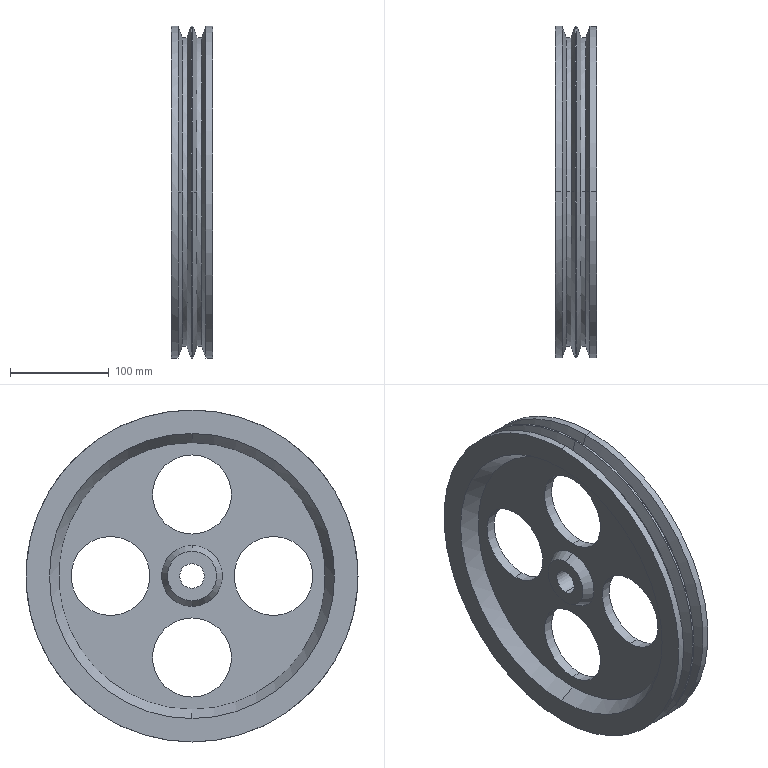Part | SolidWorks | features BaseBody 1 | 1 solid | 42 faces | box 42 x 336 x 336 mm | volume 1380304 mm3 | cylinder 20 | cone 16 | plane 6 | commonest cylinder face diameters 80 x8 336 x6 312.6 x4 25 x2
STEP:
#1=CARTESIAN_POINT('',(-5.,0.,-135.));
#2=VERTEX_POINT('',#1);
#3=CARTESIAN_POINT('',(-5.,0.,135.));
#4=VERTEX_POINT('',#3);
#5=CARTESIAN_POINT('',(-5.,0.,0.));
#6=DIRECTION('',(-1.,0.,0.));
#7=DIRECTION('',(0.,0.,1.));
#8=AXIS2_PLACEMENT_3D('',#5,#6,#7);
#9=CIRCLE('',#8,135.);
#10=EDGE_CURVE('',#2,#4,#9,.T.);
#11=ORIENTED_EDGE('',*,*,#10,.F.);
#12=CARTESIAN_POINT('',(-21.,0.,-144.238));
#13=VERTEX_POINT('',#12);
#14=CARTESIAN_POINT('',(-21.,0.,-144.238));
#15=DIRECTION('',(-0.866,0.,-0.5));
#16=VECTOR('',#15,1000.);
#17=LINE('',#14,#16);
#18=EDGE_CURVE('',#2,#13,#17,.T.);
#19=ORIENTED_EDGE('',*,*,#18,.T.);
#20=CARTESIAN_POINT('',(-21.,0.,144.238));
#21=VERTEX_POINT('',#20);
#22=CARTESIAN_POINT('',(-21.,0.,0.));
#23=DIRECTION('',(1.,0.,0.));
#24=DIRECTION('',(0.,0.,1.));
#25=AXIS2_PLACEMENT_3D('',#22,#23,#24);
#26=CIRCLE('',#25,144.238);
#27=EDGE_CURVE('',#21,#13,#26,.T.);
#28=ORIENTED_EDGE('',*,*,#27,.F.);
#29=CARTESIAN_POINT('',(-21.,0.,144.238));
#30=DIRECTION('',(-0.866,0.,0.5));
#31=VECTOR('',#30,1000.);
#32=LINE('',#29,#31);
#33=EDGE_CURVE('',#4,#21,#32,.T.);
#34=ORIENTED_EDGE('',*,*,#33,.F.);
#35=EDGE_LOOP('',(#11,#19,#28,#34));
#36=FACE_OUTER_BOUND('',#35,.T.);
#37=CARTESIAN_POINT('',(-21.,0.,0.));
#38=DIRECTION('',(-1.,0.,0.));
#39=DIRECTION('',(0.,0.,1.));
#40=AXIS2_PLACEMENT_3D('',#37,#38,#39);
#41=CONICAL_SURFACE('',#40,144.238,0.5236);
#42=ADVANCED_FACE('',(#36),#41,.F.);
#43=CARTESIAN_POINT('',(-15.,0.,-25.));
#44=VERTEX_POINT('',#43);
#45=CARTESIAN_POINT('',(-15.,0.,25.));
#46=VERTEX_POINT('',#45);
#47=CARTESIAN_POINT('',(-15.,0.,0.));
#48=DIRECTION('',(1.,0.,0.));
#49=DIRECTION('',(0.,0.,-1.));
#50=AXIS2_PLACEMENT_3D('',#47,#48,#49);
#51=CIRCLE('',#50,25.);
#52=EDGE_CURVE('',#44,#46,#51,.T.);
#53=ORIENTED_EDGE('',*,*,#52,.T.);
#54=CARTESIAN_POINT('',(-5.,0.,30.774));
#55=VERTEX_POINT('',#54);
#56=CARTESIAN_POINT('',(-5.,0.,30.774));
#57=DIRECTION('',(0.866,0.,0.5));
#58=VECTOR('',#57,1000.);
#59=LINE('',#56,#58);
#60=EDGE_CURVE('',#46,#55,#59,.T.);
#61=ORIENTED_EDGE('',*,*,#60,.T.);
#62=CARTESIAN_POINT('',(-5.,0.,-30.774));
#63=VERTEX_POINT('',#62);
#64=CARTESIAN_POINT('',(-5.,0.,0.));
#65=DIRECTION('',(1.,0.,0.));
#66=DIRECTION('',(0.,0.,-1.));
#67=AXIS2_PLACEMENT_3D('',#64,#65,#66);
#68=CIRCLE('',#67,30.774);
#69=EDGE_CURVE('',#63,#55,#68,.T.);
#70=ORIENTED_EDGE('',*,*,#69,.F.);
#71=CARTESIAN_POINT('',(-5.,0.,-30.774));
#72=DIRECTION('',(0.866,0.,-0.5));
#73=VECTOR('',#72,1000.);
#74=LINE('',#71,#73);
#75=EDGE_CURVE('',#44,#63,#74,.T.);
#76=ORIENTED_EDGE('',*,*,#75,.F.);
#77=EDGE_LOOP('',(#53,#61,#70,#76));
#78=FACE_OUTER_BOUND('',#77,.T.);
#79=CARTESIAN_POINT('',(-5.,0.,0.));
#80=DIRECTION('',(1.,0.,0.));
#81=DIRECTION('',(0.,0.,-1.));
#82=AXIS2_PLACEMENT_3D('',#79,#80,#81);
#83=CONICAL_SURFACE('',#82,30.774,0.5236);
#84=ADVANCED_FACE('',(#78),#83,.T.);
#85=CARTESIAN_POINT('',(5.,82.5,-40.));
#86=VERTEX_POINT('',#85);
#87=CARTESIAN_POINT('',(5.,82.5,40.));
#88=VERTEX_POINT('',#87);
#89=CARTESIAN_POINT('',(5.,82.5,0.));
#90=DIRECTION('',(-1.,0.,0.));
#91=DIRECTION('',(0.,0.,1.));
#92=AXIS2_PLACEMENT_3D('',#89,#90,#91);
#93=CIRCLE('',#92,40.);
#94=EDGE_CURVE('',#86,#88,#93,.T.);
#95=ORIENTED_EDGE('',*,*,#94,.F.);
#96=CARTESIAN_POINT('',(-5.,82.5,-40.));
#97=VERTEX_POINT('',#96);
#98=CARTESIAN_POINT('',(5.,82.5,-40.));
#99=DIRECTION('',(-1.,0.,0.));
#100=VECTOR('',#99,1000.);
#101=LINE('',#98,#100);
#102=EDGE_CURVE('',#86,#97,#101,.T.);
#103=ORIENTED_EDGE('',*,*,#102,.T.);
#104=CARTESIAN_POINT('',(-5.,82.5,40.));
#105=VERTEX_POINT('',#104);
#106=CARTESIAN_POINT('',(-5.,82.5,0.));
#107=DIRECTION('',(1.,0.,0.));
#108=DIRECTION('',(0.,0.,1.));
#109=AXIS2_PLACEMENT_3D('',#106,#107,#108);
#110=CIRCLE('',#109,40.);
#111=EDGE_CURVE('',#105,#97,#110,.T.);
#112=ORIENTED_EDGE('',*,*,#111,.F.);
#113=CARTESIAN_POINT('',(5.,82.5,40.));
#114=DIRECTION('',(-1.,0.,0.));
#115=VECTOR('',#114,1000.);
#116=LINE('',#113,#115);
#117=EDGE_CURVE('',#88,#105,#116,.T.);
#118=ORIENTED_EDGE('',*,*,#117,.F.);
#119=EDGE_LOOP('',(#95,#103,#112,#118));
#120=FACE_OUTER_BOUND('',#119,.T.);
#121=CARTESIAN_POINT('',(5.,82.5,0.));
#122=DIRECTION('',(-1.,0.,0.));
#123=DIRECTION('',(0.,0.,1.));
#124=AXIS2_PLACEMENT_3D('',#121,#122,#123);
#125=CYLINDRICAL_SURFACE('',#124,40.);
#126=ADVANCED_FACE('',(#120),#125,.F.);
#127=CARTESIAN_POINT('',(5.,0.,42.5));
#128=VERTEX_POINT('',#127);
#129=CARTESIAN_POINT('',(5.,0.,122.5));
#130=VERTEX_POINT('',#129);
#131=CARTESIAN_POINT('',(5.,0.,82.5));
#132=DIRECTION('',(-1.,0.,0.));
#133=DIRECTION('',(0.,0.,1.));
#134=AXIS2_PLACEMENT_3D('',#131,#132,#133);
#135=CIRCLE('',#134,40.);
#136=EDGE_CURVE('',#128,#130,#135,.T.);
#137=ORIENTED_EDGE('',*,*,#136,.F.);
#138=CARTESIAN_POINT('',(-5.,0.,42.5));
#139=VERTEX_POINT('',#138);
#140=CARTESIAN_POINT('',(5.,0.,42.5));
#141=DIRECTION('',(-1.,0.,0.));
#142=VECTOR('',#141,1000.);
#143=LINE('',#140,#142);
#144=EDGE_CURVE('',#128,#139,#143,.T.);
#145=ORIENTED_EDGE('',*,*,#144,.T.);
#146=CARTESIAN_POINT('',(-5.,0.,122.5));
#147=VERTEX_POINT('',#146);
#148=CARTESIAN_POINT('',(-5.,0.,82.5));
#149=DIRECTION('',(1.,0.,0.));
#150=DIRECTION('',(0.,0.,1.));
#151=AXIS2_PLACEMENT_3D('',#148,#149,#150);
#152=CIRCLE('',#151,40.);
#153=EDGE_CURVE('',#147,#139,#152,.T.);
#154=ORIENTED_EDGE('',*,*,#153,.F.);
#155=CARTESIAN_POINT('',(5.,0.,122.5));
#156=DIRECTION('',(-1.,0.,0.));
#157=VECTOR('',#156,1000.);
#158=LINE('',#155,#157);
#159=EDGE_CURVE('',#130,#147,#158,.T.);
#160=ORIENTED_EDGE('',*,*,#159,.F.);
#161=EDGE_LOOP('',(#137,#145,#154,#160));
#162=FACE_OUTER_BOUND('',#161,.T.);
#163=CARTESIAN_POINT('',(5.,0.,82.5));
#164=DIRECTION('',(-1.,0.,0.));
#165=DIRECTION('',(0.,0.,1.));
#166=AXIS2_PLACEMENT_3D('',#163,#164,#165);
#167=CYLINDRICAL_SURFACE('',#166,40.);
#168=ADVANCED_FACE('',(#162),#167,.F.);
#169=CARTESIAN_POINT('',(5.,-82.5,-40.));
#170=VERTEX_POINT('',#169);
#171=CARTESIAN_POINT('',(5.,-82.5,40.));
#172=VERTEX_POINT('',#171);
#173=CARTESIAN_POINT('',(5.,-82.5,0.));
#174=DIRECTION('',(-1.,0.,0.));
#175=DIRECTION('',(0.,0.,1.));
#176=AXIS2_PLACEMENT_3D('',#173,#174,#175);
#177=CIRCLE('',#176,40.);
#178=EDGE_CURVE('',#170,#172,#177,.T.);
#179=ORIENTED_EDGE('',*,*,#178,.F.);
#180=CARTESIAN_POINT('',(-5.,-82.5,-40.));
#181=VERTEX_POINT('',#180);
#182=CARTESIAN_POINT('',(5.,-82.5,-40.));
#183=DIRECTION('',(-1.,0.,0.));
#184=VECTOR('',#183,1000.);
#185=LINE('',#182,#184);
#186=EDGE_CURVE('',#170,#181,#185,.T.);
#187=ORIENTED_EDGE('',*,*,#186,.T.);
#188=CARTESIAN_POINT('',(-5.,-82.5,40.));
#189=VERTEX_POINT('',#188);
#190=CARTESIAN_POINT('',(-5.,-82.5,0.));
#191=DIRECTION('',(1.,0.,0.));
#192=DIRECTION('',(0.,0.,1.));
#193=AXIS2_PLACEMENT_3D('',#190,#191,#192);
#194=CIRCLE('',#193,40.);
#195=EDGE_CURVE('',#189,#181,#194,.T.);
#196=ORIENTED_EDGE('',*,*,#195,.F.);
#197=CARTESIAN_POINT('',(5.,-82.5,40.));
#198=DIRECTION('',(-1.,0.,0.));
#199=VECTOR('',#198,1000.);
#200=LINE('',#197,#199);
#201=EDGE_CURVE('',#172,#189,#200,.T.);
#202=ORIENTED_EDGE('',*,*,#201,.F.);
#203=EDGE_LOOP('',(#179,#187,#196,#202));
#204=FACE_OUTER_BOUND('',#203,.T.);
#205=CARTESIAN_POINT('',(5.,-82.5,0.));
#206=DIRECTION('',(-1.,0.,0.));
#207=DIRECTION('',(0.,0.,1.));
#208=AXIS2_PLACEMENT_3D('',#205,#206,#207);
#209=CYLINDRICAL_SURFACE('',#208,40.);
#210=ADVANCED_FACE('',(#204),#209,.F.);
#211=CARTESIAN_POINT('',(5.,0.,-122.5));
#212=VERTEX_POINT('',#211);
#213=CARTESIAN_POINT('',(5.,0.,-42.5));
#214=VERTEX_POINT('',#213);
#215=CARTESIAN_POINT('',(5.,0.,-82.5));
#216=DIRECTION('',(-1.,0.,0.));
#217=DIRECTION('',(0.,0.,1.));
#218=AXIS2_PLACEMENT_3D('',#215,#216,#217);
#219=CIRCLE('',#218,40.);
#220=EDGE_CURVE('',#212,#214,#219,.T.);
#221=ORIENTED_EDGE('',*,*,#220,.F.);
#222=CARTESIAN_POINT('',(-5.,0.,-122.5));
#223=VERTEX_POINT('',#222);
#224=CARTESIAN_POINT('',(5.,0.,-122.5));
#225=DIRECTION('',(-1.,0.,0.));
#226=VECTOR('',#225,1000.);
#227=LINE('',#224,#226);
#228=EDGE_CURVE('',#212,#223,#227,.T.);
#229=ORIENTED_EDGE('',*,*,#228,.T.);
#230=CARTESIAN_POINT('',(-5.,0.,-42.5));
#231=VERTEX_POINT('',#230);
#232=CARTESIAN_POINT('',(-5.,0.,-82.5));
#233=DIRECTION('',(1.,0.,0.));
#234=DIRECTION('',(0.,0.,1.));
#235=AXIS2_PLACEMENT_3D('',#232,#233,#234);
#236=CIRCLE('',#235,40.);
#237=EDGE_CURVE('',#231,#223,#236,.T.);
#238=ORIENTED_EDGE('',*,*,#237,.F.);
#239=CARTESIAN_POINT('',(5.,0.,-42.5));
#240=DIRECTION('',(-1.,0.,0.));
#241=VECTOR('',#240,1000.);
#242=LINE('',#239,#241);
#243=EDGE_CURVE('',#214,#231,#242,.T.);
#244=ORIENTED_EDGE('',*,*,#243,.F.);
#245=EDGE_LOOP('',(#221,#229,#238,#244));
#246=FACE_OUTER_BOUND('',#245,.T.);
#247=CARTESIAN_POINT('',(5.,0.,-82.5));
#248=DIRECTION('',(-1.,0.,0.));
#249=DIRECTION('',(0.,0.,1.));
#250=AXIS2_PLACEMENT_3D('',#247,#248,#249);
#251=CYLINDRICAL_SURFACE('',#250,40.);
#252=ADVANCED_FACE('',(#246),#251,.F.);
#253=CARTESIAN_POINT('',(-21.,0.,168.));
#254=VERTEX_POINT('',#253);
#255=CARTESIAN_POINT('',(-21.,0.,-168.));
#256=VERTEX_POINT('',#255);
#257=CARTESIAN_POINT('',(-21.,0.,0.));
#258=DIRECTION('',(-1.,0.,0.));
#259=DIRECTION('',(0.,0.,-1.));
#260=AXIS2_PLACEMENT_3D('',#257,#258,#259);
#261=CIRCLE('',#260,168.);
#262=EDGE_CURVE('',#254,#256,#261,.T.);
#263=ORIENTED_EDGE('',*,*,#262,.F.);
#264=CARTESIAN_POINT('',(-14.033,0.,168.));
#265=VERTEX_POINT('',#264);
#266=CARTESIAN_POINT('',(0.,0.,168.));
#267=DIRECTION('',(1.,0.,0.));
#268=VECTOR('',#267,1000.);
#269=LINE('',#266,#268);
#270=EDGE_CURVE('',#254,#265,#269,.T.);
#271=ORIENTED_EDGE('',*,*,#270,.T.);
#272=CARTESIAN_POINT('',(-14.033,168.,0.));
#273=VERTEX_POINT('',#272);
#274=CARTESIAN_POINT('',(-14.033,0.,0.));
#275=DIRECTION('',(-1.,0.,0.));
#276=DIRECTION('',(0.,0.,-1.));
#277=AXIS2_PLACEMENT_3D('',#274,#275,#276);
#278=CIRCLE('',#277,168.);
#279=EDGE_CURVE('',#265,#273,#278,.T.);
#280=ORIENTED_EDGE('',*,*,#279,.T.);
#281=CARTESIAN_POINT('',(-14.033,0.,-168.));
#282=VERTEX_POINT('',#281);
#283=CARTESIAN_POINT('',(-14.033,0.,0.));
#284=DIRECTION('',(-1.,0.,0.));
#285=DIRECTION('',(0.,0.,-1.));
#286=AXIS2_PLACEMENT_3D('',#283,#284,#285);
#287=CIRCLE('',#286,168.);
#288=EDGE_CURVE('',#273,#282,#287,.T.);
#289=ORIENTED_EDGE('',*,*,#288,.T.);
#290=CARTESIAN_POINT('',(0.,0.,-168.));
#291=DIRECTION('',(1.,0.,0.));
#292=VECTOR('',#291,1000.);
#293=LINE('',#290,#292);
#294=EDGE_CURVE('',#256,#282,#293,.T.);
#295=ORIENTED_EDGE('',*,*,#294,.F.);
#296=EDGE_LOOP('',(#263,#271,#280,#289,#295));
#297=FACE_OUTER_BOUND('',#296,.T.);
#298=CARTESIAN_POINT('',(0.,0.,0.));
#299=DIRECTION('',(1.,0.,0.));
#300=DIRECTION('',(0.,0.,-1.));
#301=AXIS2_PLACEMENT_3D('',#298,#299,#300);
#302=CYLINDRICAL_SURFACE('',#301,168.);
#303=ADVANCED_FACE('',(#297),#302,.T.);
#304=CARTESIAN_POINT('',(-15.,0.,12.5));
#305=VERTEX_POINT('',#304);
#306=CARTESIAN_POINT('',(-15.,0.,-12.5));
#307=VERTEX_POINT('',#306);
#308=CARTESIAN_POINT('',(-15.,0.,0.));
#309=DIRECTION('',(1.,0.,0.));
#310=DIRECTION('',(0.,0.,-1.));
#311=AXIS2_PLACEMENT_3D('',#308,#309,#310);
#312=CIRCLE('',#311,12.5);
#313=EDGE_CURVE('',#305,#307,#312,.T.);
#314=ORIENTED_EDGE('',*,*,#313,.F.);
#315=CARTESIAN_POINT('',(15.,0.,12.5));
#316=VERTEX_POINT('',#315);
#317=CARTESIAN_POINT('',(0.,0.,12.5));
#318=DIRECTION('',(1.,0.,0.));
#319=VECTOR('',#318,1000.);
#320=LINE('',#317,#319);
#321=EDGE_CURVE('',#305,#316,#320,.T.);
#322=ORIENTED_EDGE('',*,*,#321,.T.);
#323=CARTESIAN_POINT('',(15.,0.,-12.5));
#324=VERTEX_POINT('',#323);
#325=CARTESIAN_POINT('',(15.,0.,0.));
#326=DIRECTION('',(-1.,0.,0.));
#327=DIRECTION('',(0.,0.,-1.));
#328=AXIS2_PLACEMENT_3D('',#325,#326,#327);
#329=CIRCLE('',#328,12.5);
#330=EDGE_CURVE('',#324,#316,#329,.T.);
#331=ORIENTED_EDGE('',*,*,#330,.F.);
#332=CARTESIAN_POINT('',(0.,0.,-12.5));
#333=DIRECTION('',(1.,0.,0.));
#334=VECTOR('',#333,1000.);
#335=LINE('',#332,#334);
#336=EDGE_CURVE('',#307,#324,#335,.T.);
#337=ORIENTED_EDGE('',*,*,#336,.F.);
#338=EDGE_LOOP('',(#314,#322,#331,#337));
#339=FACE_OUTER_BOUND('',#338,.T.);
#340=CARTESIAN_POINT('',(0.,0.,0.));
#341=DIRECTION('',(1.,0.,0.));
#342=DIRECTION('',(0.,0.,-1.));
#343=AXIS2_PLACEMENT_3D('',#340,#341,#342);
#344=CYLINDRICAL_SURFACE('',#343,12.5);
#345=ADVANCED_FACE('',(#339),#344,.F.);
#346=CARTESIAN_POINT('',(15.,0.,25.));
#347=VERTEX_POINT('',#346);
#348=CARTESIAN_POINT('',(15.,0.,-25.));
#349=VERTEX_POINT('',#348);
#350=CARTESIAN_POINT('',(15.,0.,0.));
#351=DIRECTION('',(-1.,0.,0.));
#352=DIRECTION('',(0.,0.,1.));
#353=AXIS2_PLACEMENT_3D('',#350,#351,#352);
#354=CIRCLE('',#353,25.);
#355=EDGE_CURVE('',#347,#349,#354,.T.);
#356=ORIENTED_EDGE('',*,*,#355,.T.);
#357=CARTESIAN_POINT('',(5.,0.,-30.774));
#358=VERTEX_POINT('',#357);
#359=CARTESIAN_POINT('',(5.,0.,-30.774));
#360=DIRECTION('',(-0.866,0.,-0.5));
#361=VECTOR('',#360,1000.);
#362=LINE('',#359,#361);
#363=EDGE_CURVE('',#349,#358,#362,.T.);
#364=ORIENTED_EDGE('',*,*,#363,.T.);
#365=CARTESIAN_POINT('',(5.,0.,30.774));
#366=VERTEX_POINT('',#365);
#367=CARTESIAN_POINT('',(5.,0.,0.));
#368=DIRECTION('',(-1.,0.,0.));
#369=DIRECTION('',(0.,0.,1.));
#370=AXIS2_PLACEMENT_3D('',#367,#368,#369);
#371=CIRCLE('',#370,30.774);
#372=EDGE_CURVE('',#366,#358,#371,.T.);
#373=ORIENTED_EDGE('',*,*,#372,.F.);
#374=CARTESIAN_POINT('',(5.,0.,30.774));
#375=DIRECTION('',(-0.866,0.,0.5));
#376=VECTOR('',#375,1000.);
#377=LINE('',#374,#376);
#378=EDGE_CURVE('',#347,#366,#377,.T.);
#379=ORIENTED_EDGE('',*,*,#378,.F.);
#380=EDGE_LOOP('',(#356,#364,#373,#379));
#381=FACE_OUTER_BOUND('',#380,.T.);
#382=CARTESIAN_POINT('',(5.,0.,0.));
#383=DIRECTION('',(-1.,0.,0.));
#384=DIRECTION('',(0.,0.,1.));
#385=AXIS2_PLACEMENT_3D('',#382,#383,#384);
#386=CONICAL_SURFACE('',#385,30.774,0.5236);
#387=ADVANCED_FACE('',(#381),#386,.T.);
#388=CARTESIAN_POINT('',(5.,0.,135.));
#389=VERTEX_POINT('',#388);
#390=CARTESIAN_POINT('',(5.,0.,-135.));
#391=VERTEX_POINT('',#390);
#392=CARTESIAN_POINT('',(5.,0.,0.));
#393=DIRECTION('',(1.,0.,0.));
#394=DIRECTION('',(0.,0.,-1.));
#395=AXIS2_PLACEMENT_3D('',#392,#393,#394);
#396=CIRCLE('',#395,135.);
#397=EDGE_CURVE('',#389,#391,#396,.T.);
#398=ORIENTED_EDGE('',*,*,#397,.F.);
#399=CARTESIAN_POINT('',(21.,0.,144.238));
#400=VERTEX_POINT('',#399);
#401=CARTESIAN_POINT('',(21.,0.,144.238));
#402=DIRECTION('',(0.866,0.,0.5));
#403=VECTOR('',#402,1000.);
#404=LINE('',#401,#403);
#405=EDGE_CURVE('',#389,#400,#404,.T.);
#406=ORIENTED_EDGE('',*,*,#405,.T.);
#407=CARTESIAN_POINT('',(21.,0.,-144.238));
#408=VERTEX_POINT('',#407);
#409=CARTESIAN_POINT('',(21.,0.,0.));
#410=DIRECTION('',(-1.,0.,0.));
#411=DIRECTION('',(0.,0.,-1.));
#412=AXIS2_PLACEMENT_3D('',#409,#410,#411);
#413=CIRCLE('',#412,144.238);
#414=EDGE_CURVE('',#408,#400,#413,.T.);
#415=ORIENTED_EDGE('',*,*,#414,.F.);
#416=CARTESIAN_POINT('',(21.,0.,-144.238));
#417=DIRECTION('',(0.866,0.,-0.5));
#418=VECTOR('',#417,1000.);
#419=LINE('',#416,#418);
#420=EDGE_CURVE('',#391,#408,#419,.T.);
#421=ORIENTED_EDGE('',*,*,#420,.F.);
#422=EDGE_LOOP('',(#398,#406,#415,#421));
#423=FACE_OUTER_BOUND('',#422,.T.);
#424=CARTESIAN_POINT('',(21.,0.,0.));
#425=DIRECTION('',(1.,0.,0.));
#426=DIRECTION('',(0.,0.,-1.));
#427=AXIS2_PLACEMENT_3D('',#424,#425,#426);
#428=CONICAL_SURFACE('',#427,144.238,0.5236);
#429=ADVANCED_FACE('',(#423),#428,.F.);
#430=CARTESIAN_POINT('',(-10.004,0.,156.3));
#431=VERTEX_POINT('',#430);
#432=CARTESIAN_POINT('',(-10.004,156.3,0.));
#433=VERTEX_POINT('',#432);
#434=CARTESIAN_POINT('',(-10.004,0.,0.));
#435=DIRECTION('',(-1.,0.,0.));
#436=DIRECTION('',(0.,0.,1.));
#437=AXIS2_PLACEMENT_3D('',#434,#435,#436);
#438=CIRCLE('',#437,156.3);
#439=EDGE_CURVE('',#431,#433,#438,.T.);
#440=ORIENTED_EDGE('',*,*,#439,.T.);
#441=CARTESIAN_POINT('',(-14.033,168.,0.));
#442=DIRECTION('',(-0.3256,0.9455,0.));
#443=VECTOR('',#442,1000.);
#444=LINE('',#441,#443);
#445=EDGE_CURVE('',#433,#273,#444,.T.);
#446=ORIENTED_EDGE('',*,*,#445,.T.);
#447=ORIENTED_EDGE('',*,*,#279,.F.);
#448=CARTESIAN_POINT('',(-14.033,-168.,0.));
#449=VERTEX_POINT('',#448);
#450=CARTESIAN_POINT('',(-14.033,0.,0.));
#451=DIRECTION('',(-1.,0.,0.));
#452=DIRECTION('',(0.,0.,-1.));
#453=AXIS2_PLACEMENT_3D('',#450,#451,#452);
#454=CIRCLE('',#453,168.);
#455=EDGE_CURVE('',#449,#265,#454,.T.);
#456=ORIENTED_EDGE('',*,*,#455,.F.);
#457=CARTESIAN_POINT('',(-10.004,-156.3,0.));
#458=VERTEX_POINT('',#457);
#459=CARTESIAN_POINT('',(-14.033,-168.,0.));
#460=DIRECTION('',(-0.3256,-0.9455,0.));
#461=VECTOR('',#460,1000.);
#462=LINE('',#459,#461);
#463=EDGE_CURVE('',#458,#449,#462,.T.);
#464=ORIENTED_EDGE('',*,*,#463,.F.);
#465=CARTESIAN_POINT('',(-10.004,0.,0.));
#466=DIRECTION('',(-1.,0.,0.));
#467=DIRECTION('',(0.,0.,1.));
#468=AXIS2_PLACEMENT_3D('',#465,#466,#467);
#469=CIRCLE('',#468,156.3);
#470=EDGE_CURVE('',#458,#431,#469,.T.);
#471=ORIENTED_EDGE('',*,*,#470,.T.);
#472=EDGE_LOOP('',(#440,#446,#447,#456,#464,#471));
#473=FACE_OUTER_BOUND('',#472,.T.);
#474=CARTESIAN_POINT('',(-14.033,0.,0.));
#475=DIRECTION('',(-1.,0.,0.));
#476=DIRECTION('',(0.,-1.,0.));
#477=AXIS2_PLACEMENT_3D('',#474,#475,#476);
#478=CONICAL_SURFACE('',#477,168.,1.239);
#479=ADVANCED_FACE('',(#473),#478,.T.);
#480=CARTESIAN_POINT('',(-4.996,0.,156.3));
#481=VERTEX_POINT('',#480);
#482=CARTESIAN_POINT('',(-4.996,0.,-156.3));
#483=VERTEX_POINT('',#482);
#484=CARTESIAN_POINT('',(-4.996,0.,0.));
#485=DIRECTION('',(-1.,0.,0.));
#486=DIRECTION('',(0.,0.,1.));
#487=AXIS2_PLACEMENT_3D('',#484,#485,#486);
#488=CIRCLE('',#487,156.3);
#489=EDGE_CURVE('',#481,#483,#488,.T.);
#490=ORIENTED_EDGE('',*,*,#489,.T.);
#491=CARTESIAN_POINT('',(-10.004,0.,-156.3));
#492=VERTEX_POINT('',#491);
#493=CARTESIAN_POINT('',(-15.,0.,-156.3));
#494=DIRECTION('',(-1.,0.,0.));
#495=VECTOR('',#494,1000.);
#496=LINE('',#493,#495);
#497=EDGE_CURVE('',#483,#492,#496,.T.);
#498=ORIENTED_EDGE('',*,*,#497,.T.);
#499=CARTESIAN_POINT('',(-10.004,0.,0.));
#500=DIRECTION('',(-1.,0.,0.));
#501=DIRECTION('',(0.,0.,1.));
#502=AXIS2_PLACEMENT_3D('',#499,#500,#501);
#503=CIRCLE('',#502,156.3);
#504=EDGE_CURVE('',#433,#492,#503,.T.);
#505=ORIENTED_EDGE('',*,*,#504,.F.);
#506=ORIENTED_EDGE('',*,*,#439,.F.);
#507=CARTESIAN_POINT('',(-15.,0.,156.3));
#508=DIRECTION('',(-1.,0.,0.));
#509=VECTOR('',#508,1000.);
#510=LINE('',#507,#509);
#511=EDGE_CURVE('',#481,#431,#510,.T.);
#512=ORIENTED_EDGE('',*,*,#511,.F.);
#513=EDGE_LOOP('',(#490,#498,#505,#506,#512));
#514=FACE_OUTER_BOUND('',#513,.T.);
#515=CARTESIAN_POINT('',(-15.,0.,0.));
#516=DIRECTION('',(-1.,0.,0.));
#517=DIRECTION('',(0.,0.,1.));
#518=AXIS2_PLACEMENT_3D('',#515,#516,#517);
#519=CYLINDRICAL_SURFACE('',#518,156.3);
#520=ADVANCED_FACE('',(#514),#519,.T.);
#521=CARTESIAN_POINT('',(14.033,0.,-168.));
#522=VERTEX_POINT('',#521);
#523=CARTESIAN_POINT('',(14.033,0.,168.));
#524=VERTEX_POINT('',#523);
#525=CARTESIAN_POINT('',(14.033,0.,0.));
#526=DIRECTION('',(1.,0.,0.));
#527=DIRECTION('',(0.,0.,-1.));
#528=AXIS2_PLACEMENT_3D('',#525,#526,#527);
#529=CIRCLE('',#528,168.);
#530=EDGE_CURVE('',#522,#524,#529,.T.);
#531=ORIENTED_EDGE('',*,*,#530,.T.);
#532=CARTESIAN_POINT('',(21.,0.,168.));
#533=VERTEX_POINT('',#532);
#534=CARTESIAN_POINT('',(0.,0.,168.));
#535=DIRECTION('',(1.,0.,0.));
#536=VECTOR('',#535,1000.);
#537=LINE('',#534,#536);
#538=EDGE_CURVE('',#524,#533,#537,.T.);
#539=ORIENTED_EDGE('',*,*,#538,.T.);
#540=CARTESIAN_POINT('',(21.,0.,-168.));
#541=VERTEX_POINT('',#540);
#542=CARTESIAN_POINT('',(21.,0.,0.));
#543=DIRECTION('',(1.,0.,0.));
#544=DIRECTION('',(0.,0.,-1.));
#545=AXIS2_PLACEMENT_3D('',#542,#543,#544);
#546=CIRCLE('',#545,168.);
#547=EDGE_CURVE('',#541,#533,#546,.T.);
#548=ORIENTED_EDGE('',*,*,#547,.F.);
#549=CARTESIAN_POINT('',(0.,0.,-168.));
#550=DIRECTION('',(1.,0.,0.));
#551=VECTOR('',#550,1000.);
#552=LINE('',#549,#551);
#553=EDGE_CURVE('',#522,#541,#552,.T.);
#554=ORIENTED_EDGE('',*,*,#553,.F.);
#555=EDGE_LOOP('',(#531,#539,#548,#554));
#556=FACE_OUTER_BOUND('',#555,.T.);
#557=CARTESIAN_POINT('',(0.,0.,0.));
#558=DIRECTION('',(1.,0.,0.));
#559=DIRECTION('',(0.,0.,-1.));
#560=AXIS2_PLACEMENT_3D('',#557,#558,#559);
#561=CYLINDRICAL_SURFACE('',#560,168.);
#562=ADVANCED_FACE('',(#556),#561,.T.);
#563=ORIENTED_EDGE('',*,*,#489,.F.);
#564=CARTESIAN_POINT('',(-0.967,0.,168.));
#565=VERTEX_POINT('',#564);
#566=CARTESIAN_POINT('',(-0.967,0.,168.));
#567=DIRECTION('',(0.3256,0.,0.9455));
#568=VECTOR('',#567,1000.);
#569=LINE('',#566,#568);
#570=EDGE_CURVE('',#481,#565,#569,.T.);
#571=ORIENTED_EDGE('',*,*,#570,.T.);
#572=CARTESIAN_POINT('',(-0.967,0.,-168.));
#573=VERTEX_POINT('',#572);
#574=CARTESIAN_POINT('',(-0.967,0.,0.));
#575=DIRECTION('',(-1.,0.,0.));
#576=DIRECTION('',(0.,0.,-1.));
#577=AXIS2_PLACEMENT_3D('',#574,#575,#576);
#578=CIRCLE('',#577,168.);
#579=EDGE_CURVE('',#565,#573,#578,.T.);
#580=ORIENTED_EDGE('',*,*,#579,.T.);
#581=CARTESIAN_POINT('',(-0.967,0.,-168.));
#582=DIRECTION('',(0.3256,0.,-0.9455));
#583=VECTOR('',#582,1000.);
#584=LINE('',#581,#583);
#585=EDGE_CURVE('',#483,#573,#584,.T.);
#586=ORIENTED_EDGE('',*,*,#585,.F.);
#587=EDGE_LOOP('',(#563,#571,#580,#586));
#588=FACE_OUTER_BOUND('',#587,.T.);
#589=CARTESIAN_POINT('',(-0.967,0.,0.));
#590=DIRECTION('',(1.,0.,0.));
#591=DIRECTION('',(0.,0.,-1.));
#592=AXIS2_PLACEMENT_3D('',#589,#590,#591);
#593=CONICAL_SURFACE('',#592,168.,1.239);
#594=ADVANCED_FACE('',(#588),#593,.T.);
#595=CARTESIAN_POINT('',(10.004,0.,-156.3));
#596=VERTEX_POINT('',#595);
#597=CARTESIAN_POINT('',(10.004,0.,156.3));
#598=VERTEX_POINT('',#597);
#599=CARTESIAN_POINT('',(10.004,0.,0.));
#600=DIRECTION('',(1.,0.,0.));
#601=DIRECTION('',(0.,0.,-1.));
#602=AXIS2_PLACEMENT_3D('',#599,#600,#601);
#603=CIRCLE('',#602,156.3);
#604=EDGE_CURVE('',#596,#598,#603,.T.);
#605=ORIENTED_EDGE('',*,*,#604,.T.);
#606=CARTESIAN_POINT('',(14.033,0.,168.));
#607=DIRECTION('',(0.3256,0.,0.9455));
#608=VECTOR('',#607,1000.);
#609=LINE('',#606,#608);
#610=EDGE_CURVE('',#598,#524,#609,.T.);
#611=ORIENTED_EDGE('',*,*,#610,.T.);
#612=ORIENTED_EDGE('',*,*,#530,.F.);
#613=CARTESIAN_POINT('',(14.033,0.,-168.));
#614=DIRECTION('',(0.3256,0.,-0.9455));
#615=VECTOR('',#614,1000.);
#616=LINE('',#613,#615);
#617=EDGE_CURVE('',#596,#522,#616,.T.);
#618=ORIENTED_EDGE('',*,*,#617,.F.);
#619=EDGE_LOOP('',(#605,#611,#612,#618));
#620=FACE_OUTER_BOUND('',#619,.T.);
#621=CARTESIAN_POINT('',(14.033,0.,0.));
#622=DIRECTION('',(1.,0.,0.));
#623=DIRECTION('',(0.,0.,-1.));
#624=AXIS2_PLACEMENT_3D('',#621,#622,#623);
#625=CONICAL_SURFACE('',#624,168.,1.239);
#626=ADVANCED_FACE('',(#620),#625,.T.);
#627=ORIENTED_EDGE('',*,*,#579,.F.);
#628=CARTESIAN_POINT('',(0.967,0.,168.));
#629=VERTEX_POINT('',#628);
#630=CARTESIAN_POINT('',(0.,0.,168.));
#631=DIRECTION('',(1.,0.,0.));
#632=VECTOR('',#631,1000.);
#633=LINE('',#630,#632);
#634=EDGE_CURVE('',#565,#629,#633,.T.);
#635=ORIENTED_EDGE('',*,*,#634,.T.);
#636=CARTESIAN_POINT('',(0.967,168.,0.));
#637=VERTEX_POINT('',#636);
#638=CARTESIAN_POINT('',(0.967,0.,0.));
#639=DIRECTION('',(-1.,0.,0.));
#640=DIRECTION('',(0.,0.,-1.));
#641=AXIS2_PLACEMENT_3D('',#638,#639,#640);
#642=CIRCLE('',#641,168.);
#643=EDGE_CURVE('',#629,#637,#642,.T.);
#644=ORIENTED_EDGE('',*,*,#643,.T.);
#645=CARTESIAN_POINT('',(0.967,0.,-168.));
#646=VERTEX_POINT('',#645);
#647=CARTESIAN_POINT('',(0.967,0.,0.));
#648=DIRECTION('',(-1.,0.,0.));
#649=DIRECTION('',(0.,0.,-1.));
#650=AXIS2_PLACEMENT_3D('',#647,#648,#649);
#651=CIRCLE('',#650,168.);
#652=EDGE_CURVE('',#637,#646,#651,.T.);
#653=ORIENTED_EDGE('',*,*,#652,.T.);
#654=CARTESIAN_POINT('',(0.,0.,-168.));
#655=DIRECTION('',(1.,0.,0.));
#656=VECTOR('',#655,1000.);
#657=LINE('',#654,#656);
#658=EDGE_CURVE('',#573,#646,#657,.T.);
#659=ORIENTED_EDGE('',*,*,#658,.F.);
#660=EDGE_LOOP('',(#627,#635,#644,#653,#659));
#661=FACE_OUTER_BOUND('',#660,.T.);
#662=CARTESIAN_POINT('',(0.,0.,0.));
#663=DIRECTION('',(1.,0.,0.));
#664=DIRECTION('',(0.,0.,-1.));
#665=AXIS2_PLACEMENT_3D('',#662,#663,#664);
#666=CYLINDRICAL_SURFACE('',#665,168.);
#667=ADVANCED_FACE('',(#661),#666,.T.);
#668=ORIENTED_EDGE('',*,*,#604,.F.);
#669=CARTESIAN_POINT('',(4.996,0.,-156.3));
#670=VERTEX_POINT('',#669);
#671=CARTESIAN_POINT('',(0.,0.,-156.3));
#672=DIRECTION('',(-1.,0.,0.));
#673=VECTOR('',#672,1000.);
#674=LINE('',#671,#673);
#675=EDGE_CURVE('',#596,#670,#674,.T.);
#676=ORIENTED_EDGE('',*,*,#675,.T.);
#677=CARTESIAN_POINT('',(4.996,156.3,0.));
#678=VERTEX_POINT('',#677);
#679=CARTESIAN_POINT('',(4.996,0.,0.));
#680=DIRECTION('',(1.,0.,0.));
#681=DIRECTION('',(0.,0.,1.));
#682=AXIS2_PLACEMENT_3D('',#679,#680,#681);
#683=CIRCLE('',#682,156.3);
#684=EDGE_CURVE('',#670,#678,#683,.T.);
#685=ORIENTED_EDGE('',*,*,#684,.T.);
#686=CARTESIAN_POINT('',(4.996,0.,156.3));
#687=VERTEX_POINT('',#686);
#688=CARTESIAN_POINT('',(4.996,0.,0.));
#689=DIRECTION('',(1.,0.,0.));
#690=DIRECTION('',(0.,0.,1.));
#691=AXIS2_PLACEMENT_3D('',#688,#689,#690);
#692=CIRCLE('',#691,156.3);
#693=EDGE_CURVE('',#678,#687,#692,.T.);
#694=ORIENTED_EDGE('',*,*,#693,.T.);
#695=CARTESIAN_POINT('',(0.,0.,156.3));
#696=DIRECTION('',(-1.,0.,0.));
#697=VECTOR('',#696,1000.);
#698=LINE('',#695,#697);
#699=EDGE_CURVE('',#598,#687,#698,.T.);
#700=ORIENTED_EDGE('',*,*,#699,.F.);
#701=EDGE_LOOP('',(#668,#676,#685,#694,#700));
#702=FACE_OUTER_BOUND('',#701,.T.);
#703=CARTESIAN_POINT('',(0.,0.,0.));
#704=DIRECTION('',(-1.,0.,0.));
#705=DIRECTION('',(0.,0.,1.));
#706=AXIS2_PLACEMENT_3D('',#703,#704,#705);
#707=CYLINDRICAL_SURFACE('',#706,156.3);
#708=ADVANCED_FACE('',(#702),#707,.T.);
#709=ORIENTED_EDGE('',*,*,#693,.F.);
#710=CARTESIAN_POINT('',(0.967,168.,0.));
#711=DIRECTION('',(-0.3256,0.9455,0.));
#712=VECTOR('',#711,1000.);
#713=LINE('',#710,#712);
#714=EDGE_CURVE('',#678,#637,#713,.T.);
#715=ORIENTED_EDGE('',*,*,#714,.T.);
#716=ORIENTED_EDGE('',*,*,#643,.F.);
#717=CARTESIAN_POINT('',(0.967,-168.,0.));
#718=VERTEX_POINT('',#717);
#719=CARTESIAN_POINT('',(0.967,0.,0.));
#720=DIRECTION('',(-1.,0.,0.));
#721=DIRECTION('',(0.,0.,-1.));
#722=AXIS2_PLACEMENT_3D('',#719,#720,#721);
#723=CIRCLE('',#722,168.);
#724=EDGE_CURVE('',#718,#629,#723,.T.);
#725=ORIENTED_EDGE('',*,*,#724,.F.);
#726=CARTESIAN_POINT('',(4.996,-156.3,0.));
#727=VERTEX_POINT('',#726);
#728=CARTESIAN_POINT('',(0.967,-168.,0.));
#729=DIRECTION('',(-0.3256,-0.9455,0.));
#730=VECTOR('',#729,1000.);
#731=LINE('',#728,#730);
#732=EDGE_CURVE('',#727,#718,#731,.T.);
#733=ORIENTED_EDGE('',*,*,#732,.F.);
#734=CARTESIAN_POINT('',(4.996,0.,0.));
#735=DIRECTION('',(1.,0.,0.));
#736=DIRECTION('',(0.,0.,1.));
#737=AXIS2_PLACEMENT_3D('',#734,#735,#736);
#738=CIRCLE('',#737,156.3);
#739=EDGE_CURVE('',#687,#727,#738,.T.);
#740=ORIENTED_EDGE('',*,*,#739,.F.);
#741=EDGE_LOOP('',(#709,#715,#716,#725,#733,#740));
#742=FACE_OUTER_BOUND('',#741,.T.);
#743=CARTESIAN_POINT('',(0.967,0.,0.));
#744=DIRECTION('',(-1.,0.,0.));
#745=DIRECTION('',(0.,-1.,0.));
#746=AXIS2_PLACEMENT_3D('',#743,#744,#745);
#747=CONICAL_SURFACE('',#746,168.,1.239);
#748=ADVANCED_FACE('',(#742),#747,.T.);
#749=CARTESIAN_POINT('',(-5.,0.,0.));
#750=DIRECTION('',(-1.,0.,0.));
#751=DIRECTION('',(0.,0.,1.));
#752=AXIS2_PLACEMENT_3D('',#749,#750,#751);
#753=CIRCLE('',#752,135.);
#754=EDGE_CURVE('',#4,#2,#753,.T.);
#755=ORIENTED_EDGE('',*,*,#754,.T.);
#756=ORIENTED_EDGE('',*,*,#10,.T.);
#757=EDGE_LOOP('',(#755,#756));
#758=FACE_OUTER_BOUND('',#757,.T.);
#759=ORIENTED_EDGE('',*,*,#69,.T.);
#760=CARTESIAN_POINT('',(-5.,0.,0.));
#761=DIRECTION('',(1.,0.,0.));
#762=DIRECTION('',(0.,0.,-1.));
#763=AXIS2_PLACEMENT_3D('',#760,#761,#762);
#764=CIRCLE('',#763,30.774);
#765=EDGE_CURVE('',#55,#63,#764,.T.);
#766=ORIENTED_EDGE('',*,*,#765,.T.);
#767=EDGE_LOOP('',(#759,#766));
#768=FACE_BOUND('',#767,.T.);
#769=ORIENTED_EDGE('',*,*,#111,.T.);
#770=CARTESIAN_POINT('',(-5.,82.5,0.));
#771=DIRECTION('',(1.,0.,0.));
#772=DIRECTION('',(0.,0.,1.));
#773=AXIS2_PLACEMENT_3D('',#770,#771,#772);
#774=CIRCLE('',#773,40.);
#775=EDGE_CURVE('',#97,#105,#774,.T.);
#776=ORIENTED_EDGE('',*,*,#775,.T.);
#777=EDGE_LOOP('',(#769,#776));
#778=FACE_BOUND('',#777,.T.);
#779=ORIENTED_EDGE('',*,*,#153,.T.);
#780=CARTESIAN_POINT('',(-5.,0.,82.5));
#781=DIRECTION('',(1.,0.,0.));
#782=DIRECTION('',(0.,0.,1.));
#783=AXIS2_PLACEMENT_3D('',#780,#781,#782);
#784=CIRCLE('',#783,40.);
#785=EDGE_CURVE('',#139,#147,#784,.T.);
#786=ORIENTED_EDGE('',*,*,#785,.T.);
#787=EDGE_LOOP('',(#779,#786));
#788=FACE_BOUND('',#787,.T.);
#789=ORIENTED_EDGE('',*,*,#195,.T.);
#790=CARTESIAN_POINT('',(-5.,-82.5,0.));
#791=DIRECTION('',(1.,0.,0.));
#792=DIRECTION('',(0.,0.,1.));
#793=AXIS2_PLACEMENT_3D('',#790,#791,#792);
#794=CIRCLE('',#793,40.);
#795=EDGE_CURVE('',#181,#189,#794,.T.);
#796=ORIENTED_EDGE('',*,*,#795,.T.);
#797=EDGE_LOOP('',(#789,#796));
#798=FACE_BOUND('',#797,.T.);
#799=ORIENTED_EDGE('',*,*,#237,.T.);
#800=CARTESIAN_POINT('',(-5.,0.,-82.5));
#801=DIRECTION('',(1.,0.,0.));
#802=DIRECTION('',(0.,0.,1.));
#803=AXIS2_PLACEMENT_3D('',#800,#801,#802);
#804=CIRCLE('',#803,40.);
#805=EDGE_CURVE('',#223,#231,#804,.T.);
#806=ORIENTED_EDGE('',*,*,#805,.T.);
#807=EDGE_LOOP('',(#799,#806));
#808=FACE_BOUND('',#807,.T.);
#809=CARTESIAN_POINT('',(-5.,135.,0.));
#810=DIRECTION('',(-1.,0.,0.));
#811=DIRECTION('',(0.,0.,1.));
#812=AXIS2_PLACEMENT_3D('',#809,#810,#811);
#813=PLANE('',#812);
#814=ADVANCED_FACE('',(#758,#768,#778,#788,#798,#808),#813,.T.);
#815=ORIENTED_EDGE('',*,*,#18,.F.);
#816=ORIENTED_EDGE('',*,*,#754,.F.);
#817=ORIENTED_EDGE('',*,*,#33,.T.);
#818=CARTESIAN_POINT('',(-21.,0.,0.));
#819=DIRECTION('',(1.,0.,0.));
#820=DIRECTION('',(0.,0.,1.));
#821=AXIS2_PLACEMENT_3D('',#818,#819,#820);
#822=CIRCLE('',#821,144.238);
#823=EDGE_CURVE('',#13,#21,#822,.T.);
#824=ORIENTED_EDGE('',*,*,#823,.F.);
#825=EDGE_LOOP('',(#815,#816,#817,#824));
#826=FACE_OUTER_BOUND('',#825,.T.);
#827=CARTESIAN_POINT('',(-21.,0.,0.));
#828=DIRECTION('',(-1.,0.,0.));
#829=DIRECTION('',(0.,0.,1.));
#830=AXIS2_PLACEMENT_3D('',#827,#828,#829);
#831=CONICAL_SURFACE('',#830,144.238,0.5236);
#832=ADVANCED_FACE('',(#826),#831,.F.);
#833=ORIENTED_EDGE('',*,*,#60,.F.);
#834=CARTESIAN_POINT('',(-15.,0.,0.));
#835=DIRECTION('',(1.,0.,0.));
#836=DIRECTION('',(0.,0.,-1.));
#837=AXIS2_PLACEMENT_3D('',#834,#835,#836);
#838=CIRCLE('',#837,25.);
#839=EDGE_CURVE('',#46,#44,#838,.T.);
#840=ORIENTED_EDGE('',*,*,#839,.T.);
#841=ORIENTED_EDGE('',*,*,#75,.T.);
#842=ORIENTED_EDGE('',*,*,#765,.F.);
#843=EDGE_LOOP('',(#833,#840,#841,#842));
#844=FACE_OUTER_BOUND('',#843,.T.);
#845=CARTESIAN_POINT('',(-5.,0.,0.));
#846=DIRECTION('',(1.,0.,0.));
#847=DIRECTION('',(0.,0.,-1.));
#848=AXIS2_PLACEMENT_3D('',#845,#846,#847);
#849=CONICAL_SURFACE('',#848,30.774,0.5236);
#850=ADVANCED_FACE('',(#844),#849,.T.);
#851=ORIENTED_EDGE('',*,*,#102,.F.);
#852=CARTESIAN_POINT('',(5.,82.5,0.));
#853=DIRECTION('',(-1.,0.,0.));
#854=DIRECTION('',(0.,0.,1.));
#855=AXIS2_PLACEMENT_3D('',#852,#853,#854);
#856=CIRCLE('',#855,40.);
#857=EDGE_CURVE('',#88,#86,#856,.T.);
#858=ORIENTED_EDGE('',*,*,#857,.F.);
#859=ORIENTED_EDGE('',*,*,#117,.T.);
#860=ORIENTED_EDGE('',*,*,#775,.F.);
#861=EDGE_LOOP('',(#851,#858,#859,#860));
#862=FACE_OUTER_BOUND('',#861,.T.);
#863=CARTESIAN_POINT('',(5.,82.5,0.));
#864=DIRECTION('',(-1.,0.,0.));
#865=DIRECTION('',(0.,0.,1.));
#866=AXIS2_PLACEMENT_3D('',#863,#864,#865);
#867=CYLINDRICAL_SURFACE('',#866,40.);
#868=ADVANCED_FACE('',(#862),#867,.F.);
#869=ORIENTED_EDGE('',*,*,#144,.F.);
#870=CARTESIAN_POINT('',(5.,0.,82.5));
#871=DIRECTION('',(-1.,0.,0.));
#872=DIRECTION('',(0.,0.,1.));
#873=AXIS2_PLACEMENT_3D('',#870,#871,#872);
#874=CIRCLE('',#873,40.);
#875=EDGE_CURVE('',#130,#128,#874,.T.);
#876=ORIENTED_EDGE('',*,*,#875,.F.);
#877=ORIENTED_EDGE('',*,*,#159,.T.);
#878=ORIENTED_EDGE('',*,*,#785,.F.);
#879=EDGE_LOOP('',(#869,#876,#877,#878));
#880=FACE_OUTER_BOUND('',#879,.T.);
#881=CARTESIAN_POINT('',(5.,0.,82.5));
#882=DIRECTION('',(-1.,0.,0.));
#883=DIRECTION('',(0.,0.,1.));
#884=AXIS2_PLACEMENT_3D('',#881,#882,#883);
#885=CYLINDRICAL_SURFACE('',#884,40.);
#886=ADVANCED_FACE('',(#880),#885,.F.);
#887=ORIENTED_EDGE('',*,*,#186,.F.);
#888=CARTESIAN_POINT('',(5.,-82.5,0.));
#889=DIRECTION('',(-1.,0.,0.));
#890=DIRECTION('',(0.,0.,1.));
#891=AXIS2_PLACEMENT_3D('',#888,#889,#890);
#892=CIRCLE('',#891,40.);
#893=EDGE_CURVE('',#172,#170,#892,.T.);
#894=ORIENTED_EDGE('',*,*,#893,.F.);
#895=ORIENTED_EDGE('',*,*,#201,.T.);
#896=ORIENTED_EDGE('',*,*,#795,.F.);
#897=EDGE_LOOP('',(#887,#894,#895,#896));
#898=FACE_OUTER_BOUND('',#897,.T.);
#899=CARTESIAN_POINT('',(5.,-82.5,0.));
#900=DIRECTION('',(-1.,0.,0.));
#901=DIRECTION('',(0.,0.,1.));
#902=AXIS2_PLACEMENT_3D('',#899,#900,#901);
#903=CYLINDRICAL_SURFACE('',#902,40.);
#904=ADVANCED_FACE('',(#898),#903,.F.);
#905=ORIENTED_EDGE('',*,*,#228,.F.);
#906=CARTESIAN_POINT('',(5.,0.,-82.5));
#907=DIRECTION('',(-1.,0.,0.));
#908=DIRECTION('',(0.,0.,1.));
#909=AXIS2_PLACEMENT_3D('',#906,#907,#908);
#910=CIRCLE('',#909,40.);
#911=EDGE_CURVE('',#214,#212,#910,.T.);
#912=ORIENTED_EDGE('',*,*,#911,.F.);
#913=ORIENTED_EDGE('',*,*,#243,.T.);
#914=ORIENTED_EDGE('',*,*,#805,.F.);
#915=EDGE_LOOP('',(#905,#912,#913,#914));
#916=FACE_OUTER_BOUND('',#915,.T.);
#917=CARTESIAN_POINT('',(5.,0.,-82.5));
#918=DIRECTION('',(-1.,0.,0.));
#919=DIRECTION('',(0.,0.,1.));
#920=AXIS2_PLACEMENT_3D('',#917,#918,#919);
#921=CYLINDRICAL_SURFACE('',#920,40.);
#922=ADVANCED_FACE('',(#916),#921,.F.);
#923=CARTESIAN_POINT('',(-21.,0.,0.));
#924=DIRECTION('',(-1.,0.,0.));
#925=DIRECTION('',(0.,0.,-1.));
#926=AXIS2_PLACEMENT_3D('',#923,#924,#925);
#927=CIRCLE('',#926,168.);
#928=EDGE_CURVE('',#256,#254,#927,.T.);
#929=ORIENTED_EDGE('',*,*,#928,.T.);
#930=ORIENTED_EDGE('',*,*,#262,.T.);
#931=EDGE_LOOP('',(#929,#930));
#932=FACE_OUTER_BOUND('',#931,.T.);
#933=ORIENTED_EDGE('',*,*,#27,.T.);
#934=ORIENTED_EDGE('',*,*,#823,.T.);
#935=EDGE_LOOP('',(#933,#934));
#936=FACE_BOUND('',#935,.T.);
#937=CARTESIAN_POINT('',(-21.,168.,0.));
#938=DIRECTION('',(-1.,0.,0.));
#939=DIRECTION('',(0.,0.,1.));
#940=AXIS2_PLACEMENT_3D('',#937,#938,#939);
#941=PLANE('',#940);
#942=ADVANCED_FACE('',(#932,#936),#941,.T.);
#943=ORIENTED_EDGE('',*,*,#52,.F.);
#944=ORIENTED_EDGE('',*,*,#839,.F.);
#945=EDGE_LOOP('',(#943,#944));
#946=FACE_OUTER_BOUND('',#945,.T.);
#947=CARTESIAN_POINT('',(-15.,0.,0.));
#948=DIRECTION('',(1.,0.,0.));
#949=DIRECTION('',(0.,0.,-1.));
#950=AXIS2_PLACEMENT_3D('',#947,#948,#949);
#951=CIRCLE('',#950,12.5);
#952=EDGE_CURVE('',#307,#305,#951,.T.);
#953=ORIENTED_EDGE('',*,*,#952,.T.);
#954=ORIENTED_EDGE('',*,*,#313,.T.);
#955=EDGE_LOOP('',(#953,#954));
#956=FACE_BOUND('',#955,.T.);
#957=CARTESIAN_POINT('',(-15.,25.,0.));
#958=DIRECTION('',(-1.,0.,0.));
#959=DIRECTION('',(0.,0.,1.));
#960=AXIS2_PLACEMENT_3D('',#957,#958,#959);
#961=PLANE('',#960);
#962=ADVANCED_FACE('',(#946,#956),#961,.T.);
#963=ORIENTED_EDGE('',*,*,#372,.T.);
#964=CARTESIAN_POINT('',(5.,0.,0.));
#965=DIRECTION('',(-1.,0.,0.));
#966=DIRECTION('',(0.,0.,1.));
#967=AXIS2_PLACEMENT_3D('',#964,#965,#966);
#968=CIRCLE('',#967,30.774);
#969=EDGE_CURVE('',#358,#366,#968,.T.);
#970=ORIENTED_EDGE('',*,*,#969,.T.);
#971=EDGE_LOOP('',(#963,#970));
#972=FACE_BOUND('',#971,.T.);
#973=CARTESIAN_POINT('',(5.,0.,0.));
#974=DIRECTION('',(1.,0.,0.));
#975=DIRECTION('',(0.,0.,-1.));
#976=AXIS2_PLACEMENT_3D('',#973,#974,#975);
#977=CIRCLE('',#976,135.);
#978=EDGE_CURVE('',#391,#389,#977,.T.);
#979=ORIENTED_EDGE('',*,*,#978,.T.);
#980=ORIENTED_EDGE('',*,*,#397,.T.);
#981=EDGE_LOOP('',(#979,#980));
#982=FACE_OUTER_BOUND('',#981,.T.);
#983=ORIENTED_EDGE('',*,*,#857,.T.);
#984=ORIENTED_EDGE('',*,*,#94,.T.);
#985=EDGE_LOOP('',(#983,#984));
#986=FACE_BOUND('',#985,.T.);
#987=ORIENTED_EDGE('',*,*,#875,.T.);
#988=ORIENTED_EDGE('',*,*,#136,.T.);
#989=EDGE_LOOP('',(#987,#988));
#990=FACE_BOUND('',#989,.T.);
#991=ORIENTED_EDGE('',*,*,#893,.T.);
#992=ORIENTED_EDGE('',*,*,#178,.T.);
#993=EDGE_LOOP('',(#991,#992));
#994=FACE_BOUND('',#993,.T.);
#995=ORIENTED_EDGE('',*,*,#911,.T.);
#996=ORIENTED_EDGE('',*,*,#220,.T.);
#997=EDGE_LOOP('',(#995,#996));
#998=FACE_BOUND('',#997,.T.);
#999=CARTESIAN_POINT('',(5.,135.,0.));
#1000=DIRECTION('',(1.,0.,0.));
#1001=DIRECTION('',(0.,0.,-1.));
#1002=AXIS2_PLACEMENT_3D('',#999,#1000,#1001);
#1003=PLANE('',#1002);
#1004=ADVANCED_FACE('',(#972,#982,#986,#990,#994,#998),#1003,.T.);
#1005=ORIENTED_EDGE('',*,*,#270,.F.);
#1006=ORIENTED_EDGE('',*,*,#928,.F.);
#1007=ORIENTED_EDGE('',*,*,#294,.T.);
#1008=CARTESIAN_POINT('',(-14.033,0.,0.));
#1009=DIRECTION('',(-1.,0.,0.));
#1010=DIRECTION('',(0.,0.,-1.));
#1011=AXIS2_PLACEMENT_3D('',#1008,#1009,#1010);
#1012=CIRCLE('',#1011,168.);
#1013=EDGE_CURVE('',#282,#449,#1012,.T.);
#1014=ORIENTED_EDGE('',*,*,#1013,.T.);
#1015=ORIENTED_EDGE('',*,*,#455,.T.);
#1016=EDGE_LOOP('',(#1005,#1006,#1007,#1014,#1015));
#1017=FACE_OUTER_BOUND('',#1016,.T.);
#1018=CARTESIAN_POINT('',(0.,0.,0.));
#1019=DIRECTION('',(1.,0.,0.));
#1020=DIRECTION('',(0.,0.,-1.));
#1021=AXIS2_PLACEMENT_3D('',#1018,#1019,#1020);
#1022=CYLINDRICAL_SURFACE('',#1021,168.);
#1023=ADVANCED_FACE('',(#1017),#1022,.T.);
#1024=ORIENTED_EDGE('',*,*,#321,.F.);
#1025=ORIENTED_EDGE('',*,*,#952,.F.);
#1026=ORIENTED_EDGE('',*,*,#336,.T.);
#1027=CARTESIAN_POINT('',(15.,0.,0.));
#1028=DIRECTION('',(-1.,0.,0.));
#1029=DIRECTION('',(0.,0.,-1.));
#1030=AXIS2_PLACEMENT_3D('',#1027,#1028,#1029);
#1031=CIRCLE('',#1030,12.5);
#1032=EDGE_CURVE('',#316,#324,#1031,.T.);
#1033=ORIENTED_EDGE('',*,*,#1032,.F.);
#1034=EDGE_LOOP('',(#1024,#1025,#1026,#1033));
#1035=FACE_OUTER_BOUND('',#1034,.T.);
#1036=CARTESIAN_POINT('',(0.,0.,0.));
#1037=DIRECTION('',(1.,0.,0.));
#1038=DIRECTION('',(0.,0.,-1.));
#1039=AXIS2_PLACEMENT_3D('',#1036,#1037,#1038);
#1040=CYLINDRICAL_SURFACE('',#1039,12.5);
#1041=ADVANCED_FACE('',(#1035),#1040,.F.);
#1042=ORIENTED_EDGE('',*,*,#363,.F.);
#1043=CARTESIAN_POINT('',(15.,0.,0.));
#1044=DIRECTION('',(-1.,0.,0.));
#1045=DIRECTION('',(0.,0.,1.));
#1046=AXIS2_PLACEMENT_3D('',#1043,#1044,#1045);
#1047=CIRCLE('',#1046,25.);
#1048=EDGE_CURVE('',#349,#347,#1047,.T.);
#1049=ORIENTED_EDGE('',*,*,#1048,.T.);
#1050=ORIENTED_EDGE('',*,*,#378,.T.);
#1051=ORIENTED_EDGE('',*,*,#969,.F.);
#1052=EDGE_LOOP('',(#1042,#1049,#1050,#1051));
#1053=FACE_OUTER_BOUND('',#1052,.T.);
#1054=CARTESIAN_POINT('',(5.,0.,0.));
#1055=DIRECTION('',(-1.,0.,0.));
#1056=DIRECTION('',(0.,0.,1.));
#1057=AXIS2_PLACEMENT_3D('',#1054,#1055,#1056);
#1058=CONICAL_SURFACE('',#1057,30.774,0.5236);
#1059=ADVANCED_FACE('',(#1053),#1058,.T.);
#1060=ORIENTED_EDGE('',*,*,#405,.F.);
#1061=ORIENTED_EDGE('',*,*,#978,.F.);
#1062=ORIENTED_EDGE('',*,*,#420,.T.);
#1063=CARTESIAN_POINT('',(21.,0.,0.));
#1064=DIRECTION('',(-1.,0.,0.));
#1065=DIRECTION('',(0.,0.,-1.));
#1066=AXIS2_PLACEMENT_3D('',#1063,#1064,#1065);
#1067=CIRCLE('',#1066,144.238);
#1068=EDGE_CURVE('',#400,#408,#1067,.T.);
#1069=ORIENTED_EDGE('',*,*,#1068,.F.);
#1070=EDGE_LOOP('',(#1060,#1061,#1062,#1069));
#1071=FACE_OUTER_BOUND('',#1070,.T.);
#1072=CARTESIAN_POINT('',(21.,0.,0.));
#1073=DIRECTION('',(1.,0.,0.));
#1074=DIRECTION('',(0.,0.,-1.));
#1075=AXIS2_PLACEMENT_3D('',#1072,#1073,#1074);
#1076=CONICAL_SURFACE('',#1075,144.238,0.5236);
#1077=ADVANCED_FACE('',(#1071),#1076,.F.);
#1078=ORIENTED_EDGE('',*,*,#445,.F.);
#1079=ORIENTED_EDGE('',*,*,#504,.T.);
#1080=CARTESIAN_POINT('',(-10.004,0.,0.));
#1081=DIRECTION('',(-1.,0.,0.));
#1082=DIRECTION('',(0.,0.,1.));
#1083=AXIS2_PLACEMENT_3D('',#1080,#1081,#1082);
#1084=CIRCLE('',#1083,156.3);
#1085=EDGE_CURVE('',#492,#458,#1084,.T.);
#1086=ORIENTED_EDGE('',*,*,#1085,.T.);
#1087=ORIENTED_EDGE('',*,*,#463,.T.);
#1088=ORIENTED_EDGE('',*,*,#1013,.F.);
#1089=ORIENTED_EDGE('',*,*,#288,.F.);
#1090=EDGE_LOOP('',(#1078,#1079,#1086,#1087,#1088,#1089));
#1091=FACE_OUTER_BOUND('',#1090,.T.);
#1092=CARTESIAN_POINT('',(-14.033,0.,0.));
#1093=DIRECTION('',(-1.,0.,0.));
#1094=DIRECTION('',(0.,-1.,0.));
#1095=AXIS2_PLACEMENT_3D('',#1092,#1093,#1094);
#1096=CONICAL_SURFACE('',#1095,168.,1.239);
#1097=ADVANCED_FACE('',(#1091),#1096,.T.);
#1098=ORIENTED_EDGE('',*,*,#330,.T.);
#1099=ORIENTED_EDGE('',*,*,#1032,.T.);
#1100=EDGE_LOOP('',(#1098,#1099));
#1101=FACE_BOUND('',#1100,.T.);
#1102=ORIENTED_EDGE('',*,*,#355,.F.);
#1103=ORIENTED_EDGE('',*,*,#1048,.F.);
#1104=EDGE_LOOP('',(#1102,#1103));
#1105=FACE_OUTER_BOUND('',#1104,.T.);
#1106=CARTESIAN_POINT('',(15.,25.,0.));
#1107=DIRECTION('',(1.,0.,0.));
#1108=DIRECTION('',(0.,0.,-1.));
#1109=AXIS2_PLACEMENT_3D('',#1106,#1107,#1108);
#1110=PLANE('',#1109);
#1111=ADVANCED_FACE('',(#1101,#1105),#1110,.T.);
#1112=ORIENTED_EDGE('',*,*,#414,.T.);
#1113=ORIENTED_EDGE('',*,*,#1068,.T.);
#1114=EDGE_LOOP('',(#1112,#1113));
#1115=FACE_BOUND('',#1114,.T.);
#1116=ORIENTED_EDGE('',*,*,#547,.T.);
#1117=CARTESIAN_POINT('',(21.,0.,0.));
#1118=DIRECTION('',(1.,0.,0.));
#1119=DIRECTION('',(0.,0.,-1.));
#1120=AXIS2_PLACEMENT_3D('',#1117,#1118,#1119);
#1121=CIRCLE('',#1120,168.);
#1122=EDGE_CURVE('',#533,#541,#1121,.T.);
#1123=ORIENTED_EDGE('',*,*,#1122,.T.);
#1124=EDGE_LOOP('',(#1116,#1123));
#1125=FACE_OUTER_BOUND('',#1124,.T.);
#1126=CARTESIAN_POINT('',(21.,168.,0.));
#1127=DIRECTION('',(1.,0.,0.));
#1128=DIRECTION('',(0.,0.,-1.));
#1129=AXIS2_PLACEMENT_3D('',#1126,#1127,#1128);
#1130=PLANE('',#1129);
#1131=ADVANCED_FACE('',(#1115,#1125),#1130,.T.);
#1132=ORIENTED_EDGE('',*,*,#497,.F.);
#1133=CARTESIAN_POINT('',(-4.996,0.,0.));
#1134=DIRECTION('',(-1.,0.,0.));
#1135=DIRECTION('',(0.,0.,1.));
#1136=AXIS2_PLACEMENT_3D('',#1133,#1134,#1135);
#1137=CIRCLE('',#1136,156.3);
#1138=EDGE_CURVE('',#483,#481,#1137,.T.);
#1139=ORIENTED_EDGE('',*,*,#1138,.T.);
#1140=ORIENTED_EDGE('',*,*,#511,.T.);
#1141=ORIENTED_EDGE('',*,*,#470,.F.);
#1142=ORIENTED_EDGE('',*,*,#1085,.F.);
#1143=EDGE_LOOP('',(#1132,#1139,#1140,#1141,#1142));
#1144=FACE_OUTER_BOUND('',#1143,.T.);
#1145=CARTESIAN_POINT('',(-15.,0.,0.));
#1146=DIRECTION('',(-1.,0.,0.));
#1147=DIRECTION('',(0.,0.,1.));
#1148=AXIS2_PLACEMENT_3D('',#1145,#1146,#1147);
#1149=CYLINDRICAL_SURFACE('',#1148,156.3);
#1150=ADVANCED_FACE('',(#1144),#1149,.T.);
#1151=ORIENTED_EDGE('',*,*,#538,.F.);
#1152=CARTESIAN_POINT('',(14.033,0.,0.));
#1153=DIRECTION('',(1.,0.,0.));
#1154=DIRECTION('',(0.,0.,-1.));
#1155=AXIS2_PLACEMENT_3D('',#1152,#1153,#1154);
#1156=CIRCLE('',#1155,168.);
#1157=EDGE_CURVE('',#524,#522,#1156,.T.);
#1158=ORIENTED_EDGE('',*,*,#1157,.T.);
#1159=ORIENTED_EDGE('',*,*,#553,.T.);
#1160=ORIENTED_EDGE('',*,*,#1122,.F.);
#1161=EDGE_LOOP('',(#1151,#1158,#1159,#1160));
#1162=FACE_OUTER_BOUND('',#1161,.T.);
#1163=CARTESIAN_POINT('',(0.,0.,0.));
#1164=DIRECTION('',(1.,0.,0.));
#1165=DIRECTION('',(0.,0.,-1.));
#1166=AXIS2_PLACEMENT_3D('',#1163,#1164,#1165);
#1167=CYLINDRICAL_SURFACE('',#1166,168.);
#1168=ADVANCED_FACE('',(#1162),#1167,.T.);
#1169=ORIENTED_EDGE('',*,*,#570,.F.);
#1170=ORIENTED_EDGE('',*,*,#1138,.F.);
#1171=ORIENTED_EDGE('',*,*,#585,.T.);
#1172=CARTESIAN_POINT('',(-0.967,0.,0.));
#1173=DIRECTION('',(-1.,0.,0.));
#1174=DIRECTION('',(0.,0.,-1.));
#1175=AXIS2_PLACEMENT_3D('',#1172,#1173,#1174);
#1176=CIRCLE('',#1175,168.);
#1177=EDGE_CURVE('',#573,#565,#1176,.T.);
#1178=ORIENTED_EDGE('',*,*,#1177,.T.);
#1179=EDGE_LOOP('',(#1169,#1170,#1171,#1178));
#1180=FACE_OUTER_BOUND('',#1179,.T.);
#1181=CARTESIAN_POINT('',(-0.967,0.,0.));
#1182=DIRECTION('',(1.,0.,0.));
#1183=DIRECTION('',(0.,0.,-1.));
#1184=AXIS2_PLACEMENT_3D('',#1181,#1182,#1183);
#1185=CONICAL_SURFACE('',#1184,168.,1.239);
#1186=ADVANCED_FACE('',(#1180),#1185,.T.);
#1187=ORIENTED_EDGE('',*,*,#610,.F.);
#1188=CARTESIAN_POINT('',(10.004,0.,0.));
#1189=DIRECTION('',(1.,0.,0.));
#1190=DIRECTION('',(0.,0.,-1.));
#1191=AXIS2_PLACEMENT_3D('',#1188,#1189,#1190);
#1192=CIRCLE('',#1191,156.3);
#1193=EDGE_CURVE('',#598,#596,#1192,.T.);
#1194=ORIENTED_EDGE('',*,*,#1193,.T.);
#1195=ORIENTED_EDGE('',*,*,#617,.T.);
#1196=ORIENTED_EDGE('',*,*,#1157,.F.);
#1197=EDGE_LOOP('',(#1187,#1194,#1195,#1196));
#1198=FACE_OUTER_BOUND('',#1197,.T.);
#1199=CARTESIAN_POINT('',(14.033,0.,0.));
#1200=DIRECTION('',(1.,0.,0.));
#1201=DIRECTION('',(0.,0.,-1.));
#1202=AXIS2_PLACEMENT_3D('',#1199,#1200,#1201);
#1203=CONICAL_SURFACE('',#1202,168.,1.239);
#1204=ADVANCED_FACE('',(#1198),#1203,.T.);
#1205=ORIENTED_EDGE('',*,*,#634,.F.);
#1206=ORIENTED_EDGE('',*,*,#1177,.F.);
#1207=ORIENTED_EDGE('',*,*,#658,.T.);
#1208=CARTESIAN_POINT('',(0.967,0.,0.));
#1209=DIRECTION('',(-1.,0.,0.));
#1210=DIRECTION('',(0.,0.,-1.));
#1211=AXIS2_PLACEMENT_3D('',#1208,#1209,#1210);
#1212=CIRCLE('',#1211,168.);
#1213=EDGE_CURVE('',#646,#718,#1212,.T.);
#1214=ORIENTED_EDGE('',*,*,#1213,.T.);
#1215=ORIENTED_EDGE('',*,*,#724,.T.);
#1216=EDGE_LOOP('',(#1205,#1206,#1207,#1214,#1215));
#1217=FACE_OUTER_BOUND('',#1216,.T.);
#1218=CARTESIAN_POINT('',(0.,0.,0.));
#1219=DIRECTION('',(1.,0.,0.));
#1220=DIRECTION('',(0.,0.,-1.));
#1221=AXIS2_PLACEMENT_3D('',#1218,#1219,#1220);
#1222=CYLINDRICAL_SURFACE('',#1221,168.);
#1223=ADVANCED_FACE('',(#1217),#1222,.T.);
#1224=ORIENTED_EDGE('',*,*,#675,.F.);
#1225=ORIENTED_EDGE('',*,*,#1193,.F.);
#1226=ORIENTED_EDGE('',*,*,#699,.T.);
#1227=ORIENTED_EDGE('',*,*,#739,.T.);
#1228=CARTESIAN_POINT('',(4.996,0.,0.));
#1229=DIRECTION('',(1.,0.,0.));
#1230=DIRECTION('',(0.,0.,1.));
#1231=AXIS2_PLACEMENT_3D('',#1228,#1229,#1230);
#1232=CIRCLE('',#1231,156.3);
#1233=EDGE_CURVE('',#727,#670,#1232,.T.);
#1234=ORIENTED_EDGE('',*,*,#1233,.T.);
#1235=EDGE_LOOP('',(#1224,#1225,#1226,#1227,#1234));
#1236=FACE_OUTER_BOUND('',#1235,.T.);
#1237=CARTESIAN_POINT('',(0.,0.,0.));
#1238=DIRECTION('',(-1.,0.,0.));
#1239=DIRECTION('',(0.,0.,1.));
#1240=AXIS2_PLACEMENT_3D('',#1237,#1238,#1239);
#1241=CYLINDRICAL_SURFACE('',#1240,156.3);
#1242=ADVANCED_FACE('',(#1236),#1241,.T.);
#1243=ORIENTED_EDGE('',*,*,#714,.F.);
#1244=ORIENTED_EDGE('',*,*,#684,.F.);
#1245=ORIENTED_EDGE('',*,*,#1233,.F.);
#1246=ORIENTED_EDGE('',*,*,#732,.T.);
#1247=ORIENTED_EDGE('',*,*,#1213,.F.);
#1248=ORIENTED_EDGE('',*,*,#652,.F.);
#1249=EDGE_LOOP('',(#1243,#1244,#1245,#1246,#1247,#1248));
#1250=FACE_OUTER_BOUND('',#1249,.T.);
#1251=CARTESIAN_POINT('',(0.967,0.,0.));
#1252=DIRECTION('',(-1.,0.,0.));
#1253=DIRECTION('',(0.,-1.,0.));
#1254=AXIS2_PLACEMENT_3D('',#1251,#1252,#1253);
#1255=CONICAL_SURFACE('',#1254,168.,1.239);
#1256=ADVANCED_FACE('',(#1250),#1255,.T.);
#1257=CLOSED_SHELL('',(#42,#84,#126,#168,#210,#252,#303,#345,#387,#429,#479,#520,#562,#594,#626,#667,#708,#748,#814,#832,#850,#868,#886,#904,#922,#942,#962,#1004,#1023,#1041,#1059,#1077,#1097,#1111,#1131,#1150,#1168,#1186,#1204,#1223,#1242,#1256));
#1258=MANIFOLD_SOLID_BREP('',#1257);
#1259=CARTESIAN_POINT('',(0.,0.,0.));
#1260=DIRECTION('',(0.,0.,1.));
#1261=DIRECTION('',(1.,0.,0.));
#1262=AXIS2_PLACEMENT_3D('',#1259,#1260,#1261);
#1263=(LENGTH_UNIT()NAMED_UNIT(*)SI_UNIT(.MILLI.,.METRE.));
#1264=UNCERTAINTY_MEASURE_WITH_UNIT(LENGTH_MEASURE(0.00001),#1263,'','');
#1265=(NAMED_UNIT(*)PLANE_ANGLE_UNIT()SI_UNIT($,.RADIAN.));
#1266=(NAMED_UNIT(*)SI_UNIT($,.STERADIAN.)SOLID_ANGLE_UNIT());
#1267=(GEOMETRIC_REPRESENTATION_CONTEXT(3)GLOBAL_UNCERTAINTY_ASSIGNED_CONTEXT((#1264))GLOBAL_UNIT_ASSIGNED_CONTEXT((#1263,#1265,#1266))REPRESENTATION_CONTEXT('',''));
#1268=ADVANCED_BREP_SHAPE_REPRESENTATION('',(#1258,#1262),#1267);